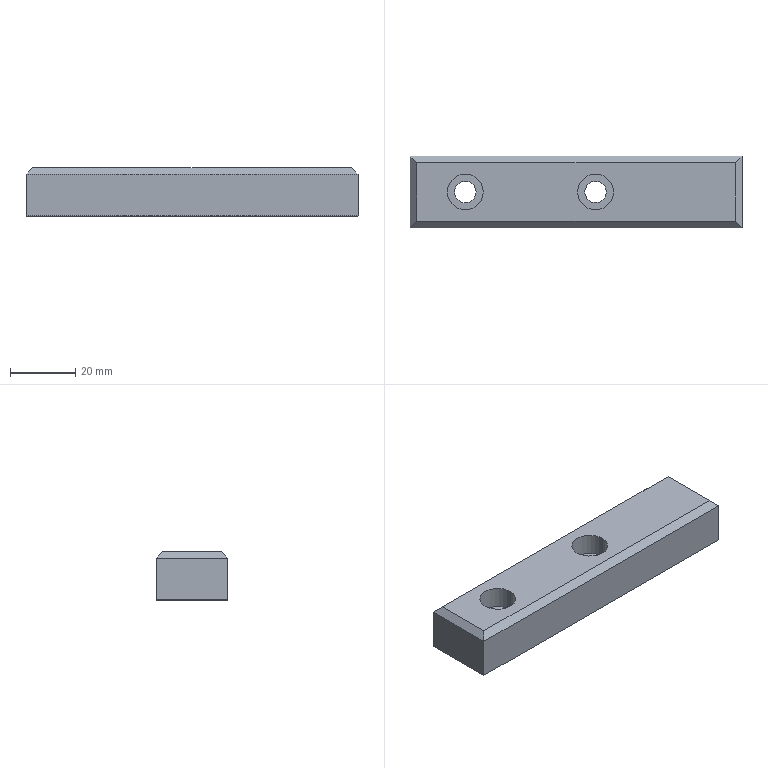Part | SolidWorks | features Chamfer 2, 3DProfileFeature 1, Extrusion 1, HoleWzd 1 | 1 solid | 24 faces | box 102 x 22 x 15 mm | volume 31316 mm3 | plane 16 | cylinder 8 | commonest cylinder face diameters 6.6 x4 11 x4
STEP:
#1=CARTESIAN_POINT('',(-39.5,0.,8.2));
#2=VERTEX_POINT('',#1);
#3=CARTESIAN_POINT('',(-28.5,0.,8.2));
#4=VERTEX_POINT('',#3);
#5=CARTESIAN_POINT('',(-34.,0.,8.2));
#6=DIRECTION('',(0.,0.,1.));
#7=DIRECTION('',(1.,0.,0.));
#8=AXIS2_PLACEMENT_3D('',#5,#6,#7);
#9=CIRCLE('',#8,5.5);
#10=EDGE_CURVE('',#2,#4,#9,.T.);
#11=ORIENTED_EDGE('',*,*,#10,.F.);
#12=CARTESIAN_POINT('',(-39.5,0.,15.));
#13=VERTEX_POINT('',#12);
#14=CARTESIAN_POINT('',(-39.5,0.,15.));
#15=DIRECTION('',(0.,0.,1.));
#16=VECTOR('',#15,1000.);
#17=LINE('',#14,#16);
#18=EDGE_CURVE('',#2,#13,#17,.T.);
#19=ORIENTED_EDGE('',*,*,#18,.T.);
#20=CARTESIAN_POINT('',(-28.5,0.,15.));
#21=VERTEX_POINT('',#20);
#22=CARTESIAN_POINT('',(-34.,0.,15.));
#23=DIRECTION('',(0.,0.,1.));
#24=DIRECTION('',(1.,0.,0.));
#25=AXIS2_PLACEMENT_3D('',#22,#23,#24);
#26=CIRCLE('',#25,5.5);
#27=EDGE_CURVE('',#13,#21,#26,.T.);
#28=ORIENTED_EDGE('',*,*,#27,.T.);
#29=CARTESIAN_POINT('',(-28.5,0.,15.));
#30=DIRECTION('',(0.,0.,1.));
#31=VECTOR('',#30,1000.);
#32=LINE('',#29,#31);
#33=EDGE_CURVE('',#4,#21,#32,.T.);
#34=ORIENTED_EDGE('',*,*,#33,.F.);
#35=EDGE_LOOP('',(#11,#19,#28,#34));
#36=FACE_OUTER_BOUND('',#35,.T.);
#37=CARTESIAN_POINT('',(-34.,0.,15.));
#38=DIRECTION('',(0.,0.,1.));
#39=DIRECTION('',(1.,0.,0.));
#40=AXIS2_PLACEMENT_3D('',#37,#38,#39);
#41=CYLINDRICAL_SURFACE('',#40,5.5);
#42=ADVANCED_FACE('',(#36),#41,.F.);
#43=CARTESIAN_POINT('',(-37.3,0.,0.));
#44=VERTEX_POINT('',#43);
#45=CARTESIAN_POINT('',(-30.7,0.,0.));
#46=VERTEX_POINT('',#45);
#47=CARTESIAN_POINT('',(-34.,0.,0.));
#48=DIRECTION('',(0.,0.,1.));
#49=DIRECTION('',(1.,0.,0.));
#50=AXIS2_PLACEMENT_3D('',#47,#48,#49);
#51=CIRCLE('',#50,3.3);
#52=EDGE_CURVE('',#44,#46,#51,.T.);
#53=ORIENTED_EDGE('',*,*,#52,.F.);
#54=CARTESIAN_POINT('',(-37.3,0.,8.2));
#55=VERTEX_POINT('',#54);
#56=CARTESIAN_POINT('',(-37.3,0.,15.));
#57=DIRECTION('',(0.,0.,1.));
#58=VECTOR('',#57,1000.);
#59=LINE('',#56,#58);
#60=EDGE_CURVE('',#44,#55,#59,.T.);
#61=ORIENTED_EDGE('',*,*,#60,.T.);
#62=CARTESIAN_POINT('',(-30.7,0.,8.2));
#63=VERTEX_POINT('',#62);
#64=CARTESIAN_POINT('',(-34.,0.,8.2));
#65=DIRECTION('',(0.,0.,1.));
#66=DIRECTION('',(1.,0.,0.));
#67=AXIS2_PLACEMENT_3D('',#64,#65,#66);
#68=CIRCLE('',#67,3.3);
#69=EDGE_CURVE('',#55,#63,#68,.T.);
#70=ORIENTED_EDGE('',*,*,#69,.T.);
#71=CARTESIAN_POINT('',(-30.7,0.,15.));
#72=DIRECTION('',(0.,0.,1.));
#73=VECTOR('',#72,1000.);
#74=LINE('',#71,#73);
#75=EDGE_CURVE('',#46,#63,#74,.T.);
#76=ORIENTED_EDGE('',*,*,#75,.F.);
#77=EDGE_LOOP('',(#53,#61,#70,#76));
#78=FACE_OUTER_BOUND('',#77,.T.);
#79=CARTESIAN_POINT('',(-34.,0.,15.));
#80=DIRECTION('',(0.,0.,1.));
#81=DIRECTION('',(1.,0.,0.));
#82=AXIS2_PLACEMENT_3D('',#79,#80,#81);
#83=CYLINDRICAL_SURFACE('',#82,3.3);
#84=ADVANCED_FACE('',(#78),#83,.F.);
#85=CARTESIAN_POINT('',(0.5,0.,8.2));
#86=VERTEX_POINT('',#85);
#87=CARTESIAN_POINT('',(11.5,0.,8.2));
#88=VERTEX_POINT('',#87);
#89=CARTESIAN_POINT('',(6.,0.,8.2));
#90=DIRECTION('',(0.,0.,1.));
#91=DIRECTION('',(1.,0.,0.));
#92=AXIS2_PLACEMENT_3D('',#89,#90,#91);
#93=CIRCLE('',#92,5.5);
#94=EDGE_CURVE('',#86,#88,#93,.T.);
#95=ORIENTED_EDGE('',*,*,#94,.F.);
#96=CARTESIAN_POINT('',(0.5,0.,15.));
#97=VERTEX_POINT('',#96);
#98=CARTESIAN_POINT('',(0.5,0.,15.));
#99=DIRECTION('',(0.,0.,1.));
#100=VECTOR('',#99,1000.);
#101=LINE('',#98,#100);
#102=EDGE_CURVE('',#86,#97,#101,.T.);
#103=ORIENTED_EDGE('',*,*,#102,.T.);
#104=CARTESIAN_POINT('',(11.5,0.,15.));
#105=VERTEX_POINT('',#104);
#106=CARTESIAN_POINT('',(6.,0.,15.));
#107=DIRECTION('',(0.,0.,1.));
#108=DIRECTION('',(1.,0.,0.));
#109=AXIS2_PLACEMENT_3D('',#106,#107,#108);
#110=CIRCLE('',#109,5.5);
#111=EDGE_CURVE('',#97,#105,#110,.T.);
#112=ORIENTED_EDGE('',*,*,#111,.T.);
#113=CARTESIAN_POINT('',(11.5,0.,15.));
#114=DIRECTION('',(0.,0.,1.));
#115=VECTOR('',#114,1000.);
#116=LINE('',#113,#115);
#117=EDGE_CURVE('',#88,#105,#116,.T.);
#118=ORIENTED_EDGE('',*,*,#117,.F.);
#119=EDGE_LOOP('',(#95,#103,#112,#118));
#120=FACE_OUTER_BOUND('',#119,.T.);
#121=CARTESIAN_POINT('',(6.,0.,15.));
#122=DIRECTION('',(0.,0.,1.));
#123=DIRECTION('',(1.,0.,0.));
#124=AXIS2_PLACEMENT_3D('',#121,#122,#123);
#125=CYLINDRICAL_SURFACE('',#124,5.5);
#126=ADVANCED_FACE('',(#120),#125,.F.);
#127=CARTESIAN_POINT('',(2.7,0.,0.));
#128=VERTEX_POINT('',#127);
#129=CARTESIAN_POINT('',(9.3,0.,0.));
#130=VERTEX_POINT('',#129);
#131=CARTESIAN_POINT('',(6.,0.,0.));
#132=DIRECTION('',(0.,0.,1.));
#133=DIRECTION('',(1.,0.,0.));
#134=AXIS2_PLACEMENT_3D('',#131,#132,#133);
#135=CIRCLE('',#134,3.3);
#136=EDGE_CURVE('',#128,#130,#135,.T.);
#137=ORIENTED_EDGE('',*,*,#136,.F.);
#138=CARTESIAN_POINT('',(2.7,0.,8.2));
#139=VERTEX_POINT('',#138);
#140=CARTESIAN_POINT('',(2.7,0.,15.));
#141=DIRECTION('',(0.,0.,1.));
#142=VECTOR('',#141,1000.);
#143=LINE('',#140,#142);
#144=EDGE_CURVE('',#128,#139,#143,.T.);
#145=ORIENTED_EDGE('',*,*,#144,.T.);
#146=CARTESIAN_POINT('',(9.3,0.,8.2));
#147=VERTEX_POINT('',#146);
#148=CARTESIAN_POINT('',(6.,0.,8.2));
#149=DIRECTION('',(0.,0.,1.));
#150=DIRECTION('',(1.,0.,0.));
#151=AXIS2_PLACEMENT_3D('',#148,#149,#150);
#152=CIRCLE('',#151,3.3);
#153=EDGE_CURVE('',#139,#147,#152,.T.);
#154=ORIENTED_EDGE('',*,*,#153,.T.);
#155=CARTESIAN_POINT('',(9.3,0.,15.));
#156=DIRECTION('',(0.,0.,1.));
#157=VECTOR('',#156,1000.);
#158=LINE('',#155,#157);
#159=EDGE_CURVE('',#130,#147,#158,.T.);
#160=ORIENTED_EDGE('',*,*,#159,.F.);
#161=EDGE_LOOP('',(#137,#145,#154,#160));
#162=FACE_OUTER_BOUND('',#161,.T.);
#163=CARTESIAN_POINT('',(6.,0.,15.));
#164=DIRECTION('',(0.,0.,1.));
#165=DIRECTION('',(1.,0.,0.));
#166=AXIS2_PLACEMENT_3D('',#163,#164,#165);
#167=CYLINDRICAL_SURFACE('',#166,3.3);
#168=ADVANCED_FACE('',(#162),#167,.F.);
#169=CARTESIAN_POINT('',(-51.,-11.,13.));
#170=VERTEX_POINT('',#169);
#171=CARTESIAN_POINT('',(-51.,-11.,0.2));
#172=VERTEX_POINT('',#171);
#173=CARTESIAN_POINT('',(-51.,-11.,15.));
#174=DIRECTION('',(0.,0.,-1.));
#175=VECTOR('',#174,1000.);
#176=LINE('',#173,#175);
#177=EDGE_CURVE('',#170,#172,#176,.T.);
#178=ORIENTED_EDGE('',*,*,#177,.F.);
#179=CARTESIAN_POINT('',(-51.,11.,13.));
#180=VERTEX_POINT('',#179);
#181=CARTESIAN_POINT('',(-51.,11.,13.));
#182=DIRECTION('',(0.,1.,0.));
#183=VECTOR('',#182,1000.);
#184=LINE('',#181,#183);
#185=EDGE_CURVE('',#170,#180,#184,.T.);
#186=ORIENTED_EDGE('',*,*,#185,.T.);
#187=CARTESIAN_POINT('',(-51.,11.,0.2));
#188=VERTEX_POINT('',#187);
#189=CARTESIAN_POINT('',(-51.,11.,15.));
#190=DIRECTION('',(0.,0.,-1.));
#191=VECTOR('',#190,1000.);
#192=LINE('',#189,#191);
#193=EDGE_CURVE('',#180,#188,#192,.T.);
#194=ORIENTED_EDGE('',*,*,#193,.T.);
#195=CARTESIAN_POINT('',(-51.,-11.,0.2));
#196=DIRECTION('',(0.,-1.,0.));
#197=VECTOR('',#196,1000.);
#198=LINE('',#195,#197);
#199=EDGE_CURVE('',#188,#172,#198,.T.);
#200=ORIENTED_EDGE('',*,*,#199,.T.);
#201=EDGE_LOOP('',(#178,#186,#194,#200));
#202=FACE_OUTER_BOUND('',#201,.T.);
#203=CARTESIAN_POINT('',(-51.,-11.,15.));
#204=DIRECTION('',(1.,0.,0.));
#205=DIRECTION('',(0.,0.,-1.));
#206=AXIS2_PLACEMENT_3D('',#203,#204,#205);
#207=PLANE('',#206);
#208=ADVANCED_FACE('',(#202),#207,.F.);
#209=CARTESIAN_POINT('',(51.,-11.,13.));
#210=VERTEX_POINT('',#209);
#211=CARTESIAN_POINT('',(51.,-11.,0.2));
#212=VERTEX_POINT('',#211);
#213=CARTESIAN_POINT('',(51.,-11.,15.));
#214=DIRECTION('',(0.,0.,-1.));
#215=VECTOR('',#214,1000.);
#216=LINE('',#213,#215);
#217=EDGE_CURVE('',#210,#212,#216,.T.);
#218=ORIENTED_EDGE('',*,*,#217,.F.);
#219=CARTESIAN_POINT('',(-51.,-11.,13.));
#220=DIRECTION('',(-1.,0.,0.));
#221=VECTOR('',#220,1000.);
#222=LINE('',#219,#221);
#223=EDGE_CURVE('',#210,#170,#222,.T.);
#224=ORIENTED_EDGE('',*,*,#223,.T.);
#225=ORIENTED_EDGE('',*,*,#177,.T.);
#226=CARTESIAN_POINT('',(51.,-11.,0.2));
#227=DIRECTION('',(1.,0.,0.));
#228=VECTOR('',#227,1000.);
#229=LINE('',#226,#228);
#230=EDGE_CURVE('',#172,#212,#229,.T.);
#231=ORIENTED_EDGE('',*,*,#230,.T.);
#232=EDGE_LOOP('',(#218,#224,#225,#231));
#233=FACE_OUTER_BOUND('',#232,.T.);
#234=CARTESIAN_POINT('',(51.,-11.,15.));
#235=DIRECTION('',(0.,1.,0.));
#236=DIRECTION('',(-1.,0.,0.));
#237=AXIS2_PLACEMENT_3D('',#234,#235,#236);
#238=PLANE('',#237);
#239=ADVANCED_FACE('',(#233),#238,.F.);
#240=CARTESIAN_POINT('',(51.,11.,13.));
#241=VERTEX_POINT('',#240);
#242=CARTESIAN_POINT('',(51.,11.,0.2));
#243=VERTEX_POINT('',#242);
#244=CARTESIAN_POINT('',(51.,11.,15.));
#245=DIRECTION('',(0.,0.,-1.));
#246=VECTOR('',#245,1000.);
#247=LINE('',#244,#246);
#248=EDGE_CURVE('',#241,#243,#247,.T.);
#249=ORIENTED_EDGE('',*,*,#248,.F.);
#250=CARTESIAN_POINT('',(51.,-11.,13.));
#251=DIRECTION('',(0.,-1.,0.));
#252=VECTOR('',#251,1000.);
#253=LINE('',#250,#252);
#254=EDGE_CURVE('',#241,#210,#253,.T.);
#255=ORIENTED_EDGE('',*,*,#254,.T.);
#256=ORIENTED_EDGE('',*,*,#217,.T.);
#257=CARTESIAN_POINT('',(51.,-11.,0.2));
#258=DIRECTION('',(0.,1.,0.));
#259=VECTOR('',#258,1000.);
#260=LINE('',#257,#259);
#261=EDGE_CURVE('',#212,#243,#260,.T.);
#262=ORIENTED_EDGE('',*,*,#261,.T.);
#263=EDGE_LOOP('',(#249,#255,#256,#262));
#264=FACE_OUTER_BOUND('',#263,.T.);
#265=CARTESIAN_POINT('',(51.,-11.,15.));
#266=DIRECTION('',(-1.,0.,0.));
#267=DIRECTION('',(0.,0.,1.));
#268=AXIS2_PLACEMENT_3D('',#265,#266,#267);
#269=PLANE('',#268);
#270=ADVANCED_FACE('',(#264),#269,.F.);
#271=ORIENTED_EDGE('',*,*,#193,.F.);
#272=CARTESIAN_POINT('',(51.,11.,13.));
#273=DIRECTION('',(1.,0.,0.));
#274=VECTOR('',#273,1000.);
#275=LINE('',#272,#274);
#276=EDGE_CURVE('',#180,#241,#275,.T.);
#277=ORIENTED_EDGE('',*,*,#276,.T.);
#278=ORIENTED_EDGE('',*,*,#248,.T.);
#279=CARTESIAN_POINT('',(51.,11.,0.2));
#280=DIRECTION('',(-1.,0.,0.));
#281=VECTOR('',#280,1000.);
#282=LINE('',#279,#281);
#283=EDGE_CURVE('',#243,#188,#282,.T.);
#284=ORIENTED_EDGE('',*,*,#283,.T.);
#285=EDGE_LOOP('',(#271,#277,#278,#284));
#286=FACE_OUTER_BOUND('',#285,.T.);
#287=CARTESIAN_POINT('',(51.,11.,15.));
#288=DIRECTION('',(0.,-1.,0.));
#289=DIRECTION('',(1.,0.,0.));
#290=AXIS2_PLACEMENT_3D('',#287,#288,#289);
#291=PLANE('',#290);
#292=ADVANCED_FACE('',(#286),#291,.F.);
#293=CARTESIAN_POINT('',(-49.,-9.,15.));
#294=VERTEX_POINT('',#293);
#295=CARTESIAN_POINT('',(49.,-9.,15.));
#296=VERTEX_POINT('',#295);
#297=CARTESIAN_POINT('',(51.,-9.,15.));
#298=DIRECTION('',(1.,0.,0.));
#299=VECTOR('',#298,1000.);
#300=LINE('',#297,#299);
#301=EDGE_CURVE('',#294,#296,#300,.T.);
#302=ORIENTED_EDGE('',*,*,#301,.T.);
#303=CARTESIAN_POINT('',(49.,9.,15.));
#304=VERTEX_POINT('',#303);
#305=CARTESIAN_POINT('',(49.,11.,15.));
#306=DIRECTION('',(0.,1.,0.));
#307=VECTOR('',#306,1000.);
#308=LINE('',#305,#307);
#309=EDGE_CURVE('',#296,#304,#308,.T.);
#310=ORIENTED_EDGE('',*,*,#309,.T.);
#311=CARTESIAN_POINT('',(-49.,9.,15.));
#312=VERTEX_POINT('',#311);
#313=CARTESIAN_POINT('',(-51.,9.,15.));
#314=DIRECTION('',(-1.,0.,0.));
#315=VECTOR('',#314,1000.);
#316=LINE('',#313,#315);
#317=EDGE_CURVE('',#304,#312,#316,.T.);
#318=ORIENTED_EDGE('',*,*,#317,.T.);
#319=CARTESIAN_POINT('',(-49.,-11.,15.));
#320=DIRECTION('',(0.,-1.,0.));
#321=VECTOR('',#320,1000.);
#322=LINE('',#319,#321);
#323=EDGE_CURVE('',#312,#294,#322,.T.);
#324=ORIENTED_EDGE('',*,*,#323,.T.);
#325=EDGE_LOOP('',(#302,#310,#318,#324));
#326=FACE_OUTER_BOUND('',#325,.T.);
#327=CARTESIAN_POINT('',(-34.,0.,15.));
#328=DIRECTION('',(0.,0.,1.));
#329=DIRECTION('',(1.,0.,0.));
#330=AXIS2_PLACEMENT_3D('',#327,#328,#329);
#331=CIRCLE('',#330,5.5);
#332=EDGE_CURVE('',#21,#13,#331,.T.);
#333=ORIENTED_EDGE('',*,*,#332,.F.);
#334=ORIENTED_EDGE('',*,*,#27,.F.);
#335=EDGE_LOOP('',(#333,#334));
#336=FACE_BOUND('',#335,.T.);
#337=CARTESIAN_POINT('',(6.,0.,15.));
#338=DIRECTION('',(0.,0.,1.));
#339=DIRECTION('',(1.,0.,0.));
#340=AXIS2_PLACEMENT_3D('',#337,#338,#339);
#341=CIRCLE('',#340,5.5);
#342=EDGE_CURVE('',#105,#97,#341,.T.);
#343=ORIENTED_EDGE('',*,*,#342,.F.);
#344=ORIENTED_EDGE('',*,*,#111,.F.);
#345=EDGE_LOOP('',(#343,#344));
#346=FACE_BOUND('',#345,.T.);
#347=CARTESIAN_POINT('',(0.,0.,15.));
#348=DIRECTION('',(0.,0.,1.));
#349=DIRECTION('',(1.,0.,0.));
#350=AXIS2_PLACEMENT_3D('',#347,#348,#349);
#351=PLANE('',#350);
#352=ADVANCED_FACE('',(#326,#336,#346),#351,.T.);
#353=CARTESIAN_POINT('',(-50.8,10.8,0.));
#354=VERTEX_POINT('',#353);
#355=CARTESIAN_POINT('',(50.8,10.8,0.));
#356=VERTEX_POINT('',#355);
#357=CARTESIAN_POINT('',(0.,10.8,0.));
#358=DIRECTION('',(1.,0.,0.));
#359=VECTOR('',#358,1000.);
#360=LINE('',#357,#359);
#361=EDGE_CURVE('',#354,#356,#360,.T.);
#362=ORIENTED_EDGE('',*,*,#361,.T.);
#363=CARTESIAN_POINT('',(50.8,-10.8,0.));
#364=VERTEX_POINT('',#363);
#365=CARTESIAN_POINT('',(50.8,0.,0.));
#366=DIRECTION('',(0.,-1.,0.));
#367=VECTOR('',#366,1000.);
#368=LINE('',#365,#367);
#369=EDGE_CURVE('',#356,#364,#368,.T.);
#370=ORIENTED_EDGE('',*,*,#369,.T.);
#371=CARTESIAN_POINT('',(-50.8,-10.8,0.));
#372=VERTEX_POINT('',#371);
#373=CARTESIAN_POINT('',(0.,-10.8,0.));
#374=DIRECTION('',(-1.,0.,0.));
#375=VECTOR('',#374,1000.);
#376=LINE('',#373,#375);
#377=EDGE_CURVE('',#364,#372,#376,.T.);
#378=ORIENTED_EDGE('',*,*,#377,.T.);
#379=CARTESIAN_POINT('',(-50.8,0.,0.));
#380=DIRECTION('',(0.,1.,0.));
#381=VECTOR('',#380,1000.);
#382=LINE('',#379,#381);
#383=EDGE_CURVE('',#372,#354,#382,.T.);
#384=ORIENTED_EDGE('',*,*,#383,.T.);
#385=EDGE_LOOP('',(#362,#370,#378,#384));
#386=FACE_OUTER_BOUND('',#385,.T.);
#387=CARTESIAN_POINT('',(-34.,0.,0.));
#388=DIRECTION('',(0.,0.,1.));
#389=DIRECTION('',(1.,0.,0.));
#390=AXIS2_PLACEMENT_3D('',#387,#388,#389);
#391=CIRCLE('',#390,3.3);
#392=EDGE_CURVE('',#46,#44,#391,.T.);
#393=ORIENTED_EDGE('',*,*,#392,.T.);
#394=ORIENTED_EDGE('',*,*,#52,.T.);
#395=EDGE_LOOP('',(#393,#394));
#396=FACE_BOUND('',#395,.T.);
#397=CARTESIAN_POINT('',(6.,0.,0.));
#398=DIRECTION('',(0.,0.,1.));
#399=DIRECTION('',(1.,0.,0.));
#400=AXIS2_PLACEMENT_3D('',#397,#398,#399);
#401=CIRCLE('',#400,3.3);
#402=EDGE_CURVE('',#130,#128,#401,.T.);
#403=ORIENTED_EDGE('',*,*,#402,.T.);
#404=ORIENTED_EDGE('',*,*,#136,.T.);
#405=EDGE_LOOP('',(#403,#404));
#406=FACE_BOUND('',#405,.T.);
#407=CARTESIAN_POINT('',(0.,0.,0.));
#408=DIRECTION('',(0.,0.,1.));
#409=DIRECTION('',(1.,0.,0.));
#410=AXIS2_PLACEMENT_3D('',#407,#408,#409);
#411=PLANE('',#410);
#412=ADVANCED_FACE('',(#386,#396,#406),#411,.F.);
#413=ORIENTED_EDGE('',*,*,#144,.F.);
#414=ORIENTED_EDGE('',*,*,#402,.F.);
#415=ORIENTED_EDGE('',*,*,#159,.T.);
#416=CARTESIAN_POINT('',(6.,0.,8.2));
#417=DIRECTION('',(0.,0.,1.));
#418=DIRECTION('',(1.,0.,0.));
#419=AXIS2_PLACEMENT_3D('',#416,#417,#418);
#420=CIRCLE('',#419,3.3);
#421=EDGE_CURVE('',#147,#139,#420,.T.);
#422=ORIENTED_EDGE('',*,*,#421,.T.);
#423=EDGE_LOOP('',(#413,#414,#415,#422));
#424=FACE_OUTER_BOUND('',#423,.T.);
#425=CARTESIAN_POINT('',(6.,0.,15.));
#426=DIRECTION('',(0.,0.,1.));
#427=DIRECTION('',(1.,0.,0.));
#428=AXIS2_PLACEMENT_3D('',#425,#426,#427);
#429=CYLINDRICAL_SURFACE('',#428,3.3);
#430=ADVANCED_FACE('',(#424),#429,.F.);
#431=ORIENTED_EDGE('',*,*,#421,.F.);
#432=ORIENTED_EDGE('',*,*,#153,.F.);
#433=EDGE_LOOP('',(#431,#432));
#434=FACE_BOUND('',#433,.T.);
#435=CARTESIAN_POINT('',(6.,0.,8.2));
#436=DIRECTION('',(0.,0.,1.));
#437=DIRECTION('',(1.,0.,0.));
#438=AXIS2_PLACEMENT_3D('',#435,#436,#437);
#439=CIRCLE('',#438,5.5);
#440=EDGE_CURVE('',#88,#86,#439,.T.);
#441=ORIENTED_EDGE('',*,*,#440,.T.);
#442=ORIENTED_EDGE('',*,*,#94,.T.);
#443=EDGE_LOOP('',(#441,#442));
#444=FACE_OUTER_BOUND('',#443,.T.);
#445=CARTESIAN_POINT('',(9.3,0.,8.2));
#446=DIRECTION('',(0.,0.,-1.));
#447=DIRECTION('',(-1.,0.,0.));
#448=AXIS2_PLACEMENT_3D('',#445,#446,#447);
#449=PLANE('',#448);
#450=ADVANCED_FACE('',(#434,#444),#449,.F.);
#451=ORIENTED_EDGE('',*,*,#102,.F.);
#452=ORIENTED_EDGE('',*,*,#440,.F.);
#453=ORIENTED_EDGE('',*,*,#117,.T.);
#454=ORIENTED_EDGE('',*,*,#342,.T.);
#455=EDGE_LOOP('',(#451,#452,#453,#454));
#456=FACE_OUTER_BOUND('',#455,.T.);
#457=CARTESIAN_POINT('',(6.,0.,15.));
#458=DIRECTION('',(0.,0.,1.));
#459=DIRECTION('',(1.,0.,0.));
#460=AXIS2_PLACEMENT_3D('',#457,#458,#459);
#461=CYLINDRICAL_SURFACE('',#460,5.5);
#462=ADVANCED_FACE('',(#456),#461,.F.);
#463=ORIENTED_EDGE('',*,*,#60,.F.);
#464=ORIENTED_EDGE('',*,*,#392,.F.);
#465=ORIENTED_EDGE('',*,*,#75,.T.);
#466=CARTESIAN_POINT('',(-34.,0.,8.2));
#467=DIRECTION('',(0.,0.,1.));
#468=DIRECTION('',(1.,0.,0.));
#469=AXIS2_PLACEMENT_3D('',#466,#467,#468);
#470=CIRCLE('',#469,3.3);
#471=EDGE_CURVE('',#63,#55,#470,.T.);
#472=ORIENTED_EDGE('',*,*,#471,.T.);
#473=EDGE_LOOP('',(#463,#464,#465,#472));
#474=FACE_OUTER_BOUND('',#473,.T.);
#475=CARTESIAN_POINT('',(-34.,0.,15.));
#476=DIRECTION('',(0.,0.,1.));
#477=DIRECTION('',(1.,0.,0.));
#478=AXIS2_PLACEMENT_3D('',#475,#476,#477);
#479=CYLINDRICAL_SURFACE('',#478,3.3);
#480=ADVANCED_FACE('',(#474),#479,.F.);
#481=ORIENTED_EDGE('',*,*,#471,.F.);
#482=ORIENTED_EDGE('',*,*,#69,.F.);
#483=EDGE_LOOP('',(#481,#482));
#484=FACE_BOUND('',#483,.T.);
#485=CARTESIAN_POINT('',(-34.,0.,8.2));
#486=DIRECTION('',(0.,0.,1.));
#487=DIRECTION('',(1.,0.,0.));
#488=AXIS2_PLACEMENT_3D('',#485,#486,#487);
#489=CIRCLE('',#488,5.5);
#490=EDGE_CURVE('',#4,#2,#489,.T.);
#491=ORIENTED_EDGE('',*,*,#490,.T.);
#492=ORIENTED_EDGE('',*,*,#10,.T.);
#493=EDGE_LOOP('',(#491,#492));
#494=FACE_OUTER_BOUND('',#493,.T.);
#495=CARTESIAN_POINT('',(-30.7,0.,8.2));
#496=DIRECTION('',(0.,0.,-1.));
#497=DIRECTION('',(-1.,0.,0.));
#498=AXIS2_PLACEMENT_3D('',#495,#496,#497);
#499=PLANE('',#498);
#500=ADVANCED_FACE('',(#484,#494),#499,.F.);
#501=ORIENTED_EDGE('',*,*,#18,.F.);
#502=ORIENTED_EDGE('',*,*,#490,.F.);
#503=ORIENTED_EDGE('',*,*,#33,.T.);
#504=ORIENTED_EDGE('',*,*,#332,.T.);
#505=EDGE_LOOP('',(#501,#502,#503,#504));
#506=FACE_OUTER_BOUND('',#505,.T.);
#507=CARTESIAN_POINT('',(-34.,0.,15.));
#508=DIRECTION('',(0.,0.,1.));
#509=DIRECTION('',(1.,0.,0.));
#510=AXIS2_PLACEMENT_3D('',#507,#508,#509);
#511=CYLINDRICAL_SURFACE('',#510,5.5);
#512=ADVANCED_FACE('',(#506),#511,.F.);
#513=CARTESIAN_POINT('',(-17.,-23.,-33.8));
#514=DIRECTION('',(-0.5774,0.5774,0.5774));
#515=VECTOR('',#514,1000.);
#516=LINE('',#513,#515);
#517=EDGE_CURVE('',#354,#188,#516,.T.);
#518=ORIENTED_EDGE('',*,*,#517,.F.);
#519=ORIENTED_EDGE('',*,*,#383,.F.);
#520=CARTESIAN_POINT('',(-51.,-11.,0.2));
#521=DIRECTION('',(0.5774,0.5774,-0.5774));
#522=VECTOR('',#521,1000.);
#523=LINE('',#520,#522);
#524=EDGE_CURVE('',#172,#372,#523,.T.);
#525=ORIENTED_EDGE('',*,*,#524,.F.);
#526=ORIENTED_EDGE('',*,*,#199,.F.);
#527=EDGE_LOOP('',(#518,#519,#525,#526));
#528=FACE_OUTER_BOUND('',#527,.T.);
#529=CARTESIAN_POINT('',(-51.,-11.,0.2));
#530=DIRECTION('',(0.7071,0.,0.7071));
#531=DIRECTION('',(0.,-1.,0.));
#532=AXIS2_PLACEMENT_3D('',#529,#530,#531);
#533=PLANE('',#532);
#534=ADVANCED_FACE('',(#528),#533,.F.);
#535=ORIENTED_EDGE('',*,*,#524,.T.);
#536=ORIENTED_EDGE('',*,*,#377,.F.);
#537=CARTESIAN_POINT('',(51.,-11.,0.2));
#538=DIRECTION('',(-0.5774,0.5774,-0.5774));
#539=VECTOR('',#538,1000.);
#540=LINE('',#537,#539);
#541=EDGE_CURVE('',#212,#364,#540,.T.);
#542=ORIENTED_EDGE('',*,*,#541,.F.);
#543=ORIENTED_EDGE('',*,*,#230,.F.);
#544=EDGE_LOOP('',(#535,#536,#542,#543));
#545=FACE_OUTER_BOUND('',#544,.T.);
#546=CARTESIAN_POINT('',(51.,-11.,0.2));
#547=DIRECTION('',(0.,0.7071,0.7071));
#548=DIRECTION('',(1.,0.,0.));
#549=AXIS2_PLACEMENT_3D('',#546,#547,#548);
#550=PLANE('',#549);
#551=ADVANCED_FACE('',(#545),#550,.F.);
#552=ORIENTED_EDGE('',*,*,#517,.T.);
#553=ORIENTED_EDGE('',*,*,#283,.F.);
#554=CARTESIAN_POINT('',(51.,11.,0.2));
#555=DIRECTION('',(0.5774,0.5774,0.5774));
#556=VECTOR('',#555,1000.);
#557=LINE('',#554,#556);
#558=EDGE_CURVE('',#356,#243,#557,.T.);
#559=ORIENTED_EDGE('',*,*,#558,.F.);
#560=ORIENTED_EDGE('',*,*,#361,.F.);
#561=EDGE_LOOP('',(#552,#553,#559,#560));
#562=FACE_OUTER_BOUND('',#561,.T.);
#563=CARTESIAN_POINT('',(51.,11.,0.2));
#564=DIRECTION('',(0.,-0.7071,0.7071));
#565=DIRECTION('',(-1.,0.,0.));
#566=AXIS2_PLACEMENT_3D('',#563,#564,#565);
#567=PLANE('',#566);
#568=ADVANCED_FACE('',(#562),#567,.F.);
#569=ORIENTED_EDGE('',*,*,#541,.T.);
#570=ORIENTED_EDGE('',*,*,#369,.F.);
#571=ORIENTED_EDGE('',*,*,#558,.T.);
#572=ORIENTED_EDGE('',*,*,#261,.F.);
#573=EDGE_LOOP('',(#569,#570,#571,#572));
#574=FACE_OUTER_BOUND('',#573,.T.);
#575=CARTESIAN_POINT('',(51.,-11.,0.2));
#576=DIRECTION('',(-0.7071,0.,0.7071));
#577=DIRECTION('',(0.,1.,0.));
#578=AXIS2_PLACEMENT_3D('',#575,#576,#577);
#579=PLANE('',#578);
#580=ADVANCED_FACE('',(#574),#579,.F.);
#581=CARTESIAN_POINT('',(-32.667,-7.333,31.333));
#582=DIRECTION('',(0.5774,-0.5774,0.5774));
#583=VECTOR('',#582,1000.);
#584=LINE('',#581,#583);
#585=EDGE_CURVE('',#180,#312,#584,.T.);
#586=ORIENTED_EDGE('',*,*,#585,.F.);
#587=ORIENTED_EDGE('',*,*,#185,.F.);
#588=CARTESIAN_POINT('',(-46.,-6.,18.));
#589=DIRECTION('',(-0.5774,-0.5774,-0.5774));
#590=VECTOR('',#589,1000.);
#591=LINE('',#588,#590);
#592=EDGE_CURVE('',#294,#170,#591,.T.);
#593=ORIENTED_EDGE('',*,*,#592,.F.);
#594=ORIENTED_EDGE('',*,*,#323,.F.);
#595=EDGE_LOOP('',(#586,#587,#593,#594));
#596=FACE_OUTER_BOUND('',#595,.T.);
#597=CARTESIAN_POINT('',(-49.,0.,15.));
#598=DIRECTION('',(-0.7071,0.,0.7071));
#599=DIRECTION('',(0.,1.,0.));
#600=AXIS2_PLACEMENT_3D('',#597,#598,#599);
#601=PLANE('',#600);
#602=ADVANCED_FACE('',(#596),#601,.T.);
#603=ORIENTED_EDGE('',*,*,#592,.T.);
#604=ORIENTED_EDGE('',*,*,#223,.F.);
#605=CARTESIAN_POINT('',(32.667,7.333,31.333));
#606=DIRECTION('',(0.5774,-0.5774,-0.5774));
#607=VECTOR('',#606,1000.);
#608=LINE('',#605,#607);
#609=EDGE_CURVE('',#296,#210,#608,.T.);
#610=ORIENTED_EDGE('',*,*,#609,.F.);
#611=ORIENTED_EDGE('',*,*,#301,.F.);
#612=EDGE_LOOP('',(#603,#604,#610,#611));
#613=FACE_OUTER_BOUND('',#612,.T.);
#614=CARTESIAN_POINT('',(0.,-9.,15.));
#615=DIRECTION('',(0.,-0.7071,0.7071));
#616=DIRECTION('',(-1.,0.,0.));
#617=AXIS2_PLACEMENT_3D('',#614,#615,#616);
#618=PLANE('',#617);
#619=ADVANCED_FACE('',(#613),#618,.T.);
#620=ORIENTED_EDGE('',*,*,#585,.T.);
#621=ORIENTED_EDGE('',*,*,#317,.F.);
#622=CARTESIAN_POINT('',(32.667,-7.333,31.333));
#623=DIRECTION('',(-0.5774,-0.5774,0.5774));
#624=VECTOR('',#623,1000.);
#625=LINE('',#622,#624);
#626=EDGE_CURVE('',#241,#304,#625,.T.);
#627=ORIENTED_EDGE('',*,*,#626,.F.);
#628=ORIENTED_EDGE('',*,*,#276,.F.);
#629=EDGE_LOOP('',(#620,#621,#627,#628));
#630=FACE_OUTER_BOUND('',#629,.T.);
#631=CARTESIAN_POINT('',(0.,9.,15.));
#632=DIRECTION('',(0.,0.7071,0.7071));
#633=DIRECTION('',(1.,0.,0.));
#634=AXIS2_PLACEMENT_3D('',#631,#632,#633);
#635=PLANE('',#634);
#636=ADVANCED_FACE('',(#630),#635,.T.);
#637=ORIENTED_EDGE('',*,*,#609,.T.);
#638=ORIENTED_EDGE('',*,*,#254,.F.);
#639=ORIENTED_EDGE('',*,*,#626,.T.);
#640=ORIENTED_EDGE('',*,*,#309,.F.);
#641=EDGE_LOOP('',(#637,#638,#639,#640));
#642=FACE_OUTER_BOUND('',#641,.T.);
#643=CARTESIAN_POINT('',(49.,0.,15.));
#644=DIRECTION('',(0.7071,0.,0.7071));
#645=DIRECTION('',(0.,-1.,0.));
#646=AXIS2_PLACEMENT_3D('',#643,#644,#645);
#647=PLANE('',#646);
#648=ADVANCED_FACE('',(#642),#647,.T.);
#649=CLOSED_SHELL('',(#42,#84,#126,#168,#208,#239,#270,#292,#352,#412,#430,#450,#462,#480,#500,#512,#534,#551,#568,#580,#602,#619,#636,#648));
#650=MANIFOLD_SOLID_BREP('',#649);
#651=CARTESIAN_POINT('',(0.,0.,0.));
#652=DIRECTION('',(0.,0.,1.));
#653=DIRECTION('',(1.,0.,0.));
#654=AXIS2_PLACEMENT_3D('',#651,#652,#653);
#655=(LENGTH_UNIT()NAMED_UNIT(*)SI_UNIT(.MILLI.,.METRE.));
#656=UNCERTAINTY_MEASURE_WITH_UNIT(LENGTH_MEASURE(0.00001),#655,'','');
#657=(NAMED_UNIT(*)PLANE_ANGLE_UNIT()SI_UNIT($,.RADIAN.));
#658=(NAMED_UNIT(*)SI_UNIT($,.STERADIAN.)SOLID_ANGLE_UNIT());
#659=(GEOMETRIC_REPRESENTATION_CONTEXT(3)GLOBAL_UNCERTAINTY_ASSIGNED_CONTEXT((#656))GLOBAL_UNIT_ASSIGNED_CONTEXT((#655,#657,#658))REPRESENTATION_CONTEXT('',''));
#660=ADVANCED_BREP_SHAPE_REPRESENTATION('',(#650,#654),#659);